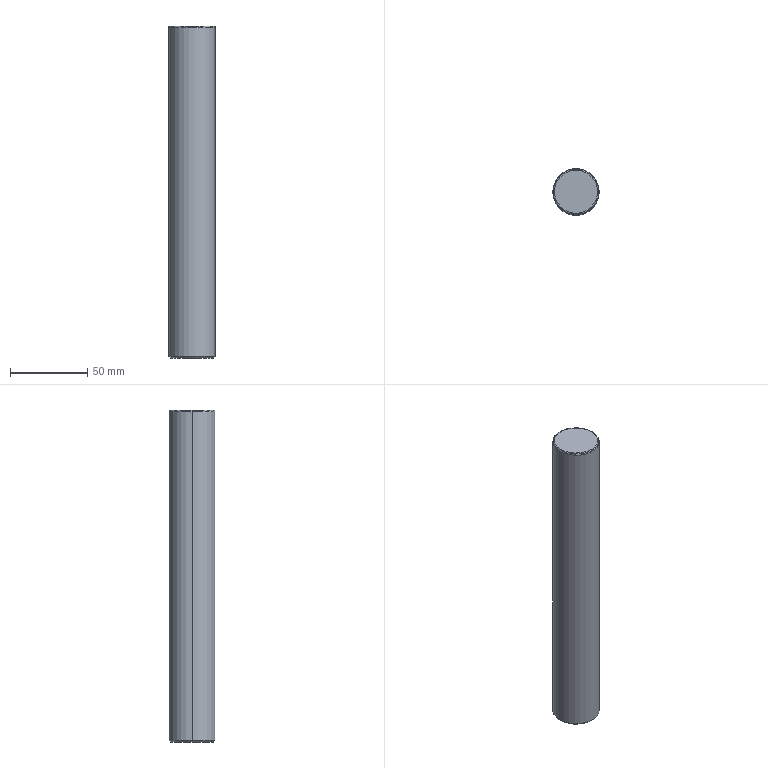Part | Creo | 1 solid | 14 faces | box 30 x 30 x 215 mm | volume 151193 mm3 | cone 4 | cylinder 4 | torus 4 | plane 2 | commonest cylinder face diameters 6.8 x2 30 x2
STEP:
#1=CARTESIAN_POINT('',(-69.,10.,-300.5));
#2=VERTEX_POINT('',#1);
#3=CARTESIAN_POINT('',(-41.,10.,-300.5));
#4=VERTEX_POINT('',#3);
#5=CARTESIAN_POINT('',(-55.,10.,-300.5));
#6=DIRECTION('',(0.,0.,-1.));
#7=DIRECTION('',(-1.,0.,0.));
#8=AXIS2_PLACEMENT_3D('',#5,#6,#7);
#9=CIRCLE('',#8,14.);
#10=EDGE_CURVE('',#2,#4,#9,.T.);
#11=ORIENTED_EDGE('',*,*,#10,.F.);
#12=CARTESIAN_POINT('',(-55.,10.,-300.5));
#13=DIRECTION('',(0.,0.,-1.));
#14=DIRECTION('',(1.,0.,0.));
#15=AXIS2_PLACEMENT_3D('',#12,#13,#14);
#16=CIRCLE('',#15,14.);
#17=EDGE_CURVE('',#4,#2,#16,.T.);
#18=ORIENTED_EDGE('',*,*,#17,.F.);
#19=EDGE_LOOP('',(#11,#18));
#20=FACE_OUTER_BOUND('',#19,.F.);
#21=CARTESIAN_POINT('',(-51.6,10.,-300.5));
#22=VERTEX_POINT('',#21);
#23=CARTESIAN_POINT('',(-58.4,10.,-300.5));
#24=VERTEX_POINT('',#23);
#25=CARTESIAN_POINT('',(-55.,10.,-300.5));
#26=DIRECTION('',(0.,0.,1.));
#27=DIRECTION('',(1.,0.,0.));
#28=AXIS2_PLACEMENT_3D('',#25,#26,#27);
#29=CIRCLE('',#28,3.4);
#30=EDGE_CURVE('',#22,#24,#29,.T.);
#31=ORIENTED_EDGE('',*,*,#30,.F.);
#32=CARTESIAN_POINT('',(-55.,10.,-300.5));
#33=DIRECTION('',(0.,0.,1.));
#34=DIRECTION('',(-1.,0.,0.));
#35=AXIS2_PLACEMENT_3D('',#32,#33,#34);
#36=CIRCLE('',#35,3.4);
#37=EDGE_CURVE('',#24,#22,#36,.T.);
#38=ORIENTED_EDGE('',*,*,#37,.F.);
#39=EDGE_LOOP('',(#31,#38));
#40=FACE_BOUND('',#39,.F.);
#41=CARTESIAN_POINT('',(-55.,10.,-300.5));
#42=DIRECTION('',(0.,0.,-1.));
#43=DIRECTION('',(-1.,0.,0.));
#44=AXIS2_PLACEMENT_3D('',#41,#42,#43);
#45=PLANE('',#44);
#46=ADVANCED_FACE('',(#20,#40),#45,.T.);
#47=ORIENTED_EDGE('',*,*,#10,.T.);
#48=CARTESIAN_POINT('',(-40.,10.,-299.5));
#49=VERTEX_POINT('',#48);
#50=CARTESIAN_POINT('',(-41.,10.,-300.5));
#51=DIRECTION('',(0.7071,0.,0.7071));
#52=VECTOR('',#51,1.414);
#53=LINE('',#50,#52);
#54=EDGE_CURVE('',#4,#49,#53,.T.);
#55=ORIENTED_EDGE('',*,*,#54,.T.);
#56=CARTESIAN_POINT('',(-70.,10.,-299.5));
#57=VERTEX_POINT('',#56);
#58=CARTESIAN_POINT('',(-55.,10.,-299.5));
#59=DIRECTION('',(0.,0.,-1.));
#60=DIRECTION('',(-1.,0.,0.));
#61=AXIS2_PLACEMENT_3D('',#58,#59,#60);
#62=CIRCLE('',#61,15.);
#63=EDGE_CURVE('',#57,#49,#62,.T.);
#64=ORIENTED_EDGE('',*,*,#63,.F.);
#65=CARTESIAN_POINT('',(-69.,10.,-300.5));
#66=DIRECTION('',(-0.7071,0.,0.7071));
#67=VECTOR('',#66,1.414);
#68=LINE('',#65,#67);
#69=EDGE_CURVE('',#2,#57,#68,.T.);
#70=ORIENTED_EDGE('',*,*,#69,.F.);
#71=EDGE_LOOP('',(#47,#55,#64,#70));
#72=FACE_OUTER_BOUND('',#71,.F.);
#73=CARTESIAN_POINT('',(-55.,10.,-300.));
#74=DIRECTION('',(0.,0.,1.));
#75=DIRECTION('',(1.,0.,0.));
#76=AXIS2_PLACEMENT_3D('',#73,#74,#75);
#77=CONICAL_SURFACE('',#76,14.5,45.);
#78=ADVANCED_FACE('',(#72),#77,.T.);
#79=ORIENTED_EDGE('',*,*,#17,.T.);
#80=ORIENTED_EDGE('',*,*,#69,.T.);
#81=CARTESIAN_POINT('',(-55.,10.,-299.5));
#82=DIRECTION('',(0.,0.,-1.));
#83=DIRECTION('',(1.,0.,0.));
#84=AXIS2_PLACEMENT_3D('',#81,#82,#83);
#85=CIRCLE('',#84,15.);
#86=EDGE_CURVE('',#49,#57,#85,.T.);
#87=ORIENTED_EDGE('',*,*,#86,.F.);
#88=ORIENTED_EDGE('',*,*,#54,.F.);
#89=EDGE_LOOP('',(#79,#80,#87,#88));
#90=FACE_OUTER_BOUND('',#89,.F.);
#91=CARTESIAN_POINT('',(-55.,10.,-300.));
#92=DIRECTION('',(0.,0.,1.));
#93=DIRECTION('',(1.,0.,0.));
#94=AXIS2_PLACEMENT_3D('',#91,#92,#93);
#95=CONICAL_SURFACE('',#94,14.5,45.);
#96=ADVANCED_FACE('',(#90),#95,.T.);
#97=ORIENTED_EDGE('',*,*,#86,.T.);
#98=CARTESIAN_POINT('',(-70.,10.,-86.5));
#99=VERTEX_POINT('',#98);
#100=CARTESIAN_POINT('',(-70.,10.,-86.5));
#101=DIRECTION('',(0.,0.,-1.));
#102=VECTOR('',#101,213.);
#103=LINE('',#100,#102);
#104=EDGE_CURVE('',#99,#57,#103,.T.);
#105=ORIENTED_EDGE('',*,*,#104,.F.);
#106=CARTESIAN_POINT('',(-40.,10.,-86.5));
#107=VERTEX_POINT('',#106);
#108=CARTESIAN_POINT('',(-55.,10.,-86.5));
#109=DIRECTION('',(0.,0.,1.));
#110=DIRECTION('',(-1.,0.,0.));
#111=AXIS2_PLACEMENT_3D('',#108,#109,#110);
#112=CIRCLE('',#111,15.);
#113=EDGE_CURVE('',#99,#107,#112,.T.);
#114=ORIENTED_EDGE('',*,*,#113,.T.);
#115=CARTESIAN_POINT('',(-40.,10.,-86.5));
#116=DIRECTION('',(0.,0.,-1.));
#117=VECTOR('',#116,213.);
#118=LINE('',#115,#117);
#119=EDGE_CURVE('',#107,#49,#118,.T.);
#120=ORIENTED_EDGE('',*,*,#119,.T.);
#121=EDGE_LOOP('',(#97,#105,#114,#120));
#122=FACE_OUTER_BOUND('',#121,.F.);
#123=CARTESIAN_POINT('',(-55.,10.,-100.5));
#124=DIRECTION('',(0.,0.,-1.));
#125=DIRECTION('',(-1.,0.,0.));
#126=AXIS2_PLACEMENT_3D('',#123,#124,#125);
#127=CYLINDRICAL_SURFACE('',#126,15.);
#128=ADVANCED_FACE('',(#122),#127,.T.);
#129=ORIENTED_EDGE('',*,*,#63,.T.);
#130=ORIENTED_EDGE('',*,*,#119,.F.);
#131=CARTESIAN_POINT('',(-55.,10.,-86.5));
#132=DIRECTION('',(0.,0.,1.));
#133=DIRECTION('',(1.,0.,0.));
#134=AXIS2_PLACEMENT_3D('',#131,#132,#133);
#135=CIRCLE('',#134,15.);
#136=EDGE_CURVE('',#107,#99,#135,.T.);
#137=ORIENTED_EDGE('',*,*,#136,.T.);
#138=ORIENTED_EDGE('',*,*,#104,.T.);
#139=EDGE_LOOP('',(#129,#130,#137,#138));
#140=FACE_OUTER_BOUND('',#139,.F.);
#141=CARTESIAN_POINT('',(-55.,10.,-100.5));
#142=DIRECTION('',(0.,0.,-1.));
#143=DIRECTION('',(-1.,0.,0.));
#144=AXIS2_PLACEMENT_3D('',#141,#142,#143);
#145=CYLINDRICAL_SURFACE('',#144,15.);
#146=ADVANCED_FACE('',(#140),#145,.T.);
#147=ORIENTED_EDGE('',*,*,#136,.F.);
#148=CARTESIAN_POINT('',(-40.293,10.,-85.793));
#149=VERTEX_POINT('',#148);
#150=CARTESIAN_POINT('',(-41.,10.,-86.5));
#151=DIRECTION('',(0.,-1.,0.));
#152=DIRECTION('',(1.,0.,0.));
#153=AXIS2_PLACEMENT_3D('',#150,#151,#152);
#154=CIRCLE('',#153,1.);
#155=EDGE_CURVE('',#107,#149,#154,.T.);
#156=ORIENTED_EDGE('',*,*,#155,.T.);
#157=CARTESIAN_POINT('',(-69.707,10.,-85.793));
#158=VERTEX_POINT('',#157);
#159=CARTESIAN_POINT('',(-55.,10.,-85.793));
#160=DIRECTION('',(0.,0.,1.));
#161=DIRECTION('',(1.,0.,0.));
#162=AXIS2_PLACEMENT_3D('',#159,#160,#161);
#163=CIRCLE('',#162,14.707);
#164=EDGE_CURVE('',#149,#158,#163,.T.);
#165=ORIENTED_EDGE('',*,*,#164,.T.);
#166=CARTESIAN_POINT('',(-69.,10.,-86.5));
#167=DIRECTION('',(0.,1.,0.));
#168=DIRECTION('',(-1.,0.,0.));
#169=AXIS2_PLACEMENT_3D('',#166,#167,#168);
#170=CIRCLE('',#169,1.);
#171=EDGE_CURVE('',#99,#158,#170,.T.);
#172=ORIENTED_EDGE('',*,*,#171,.F.);
#173=EDGE_LOOP('',(#147,#156,#165,#172));
#174=FACE_OUTER_BOUND('',#173,.F.);
#175=CARTESIAN_POINT('',(-55.,10.,-86.5));
#176=DIRECTION('',(0.,0.,1.));
#177=DIRECTION('',(1.,0.,0.));
#178=AXIS2_PLACEMENT_3D('',#175,#176,#177);
#179=TOROIDAL_SURFACE('',#178,14.,1.);
#180=ADVANCED_FACE('',(#174),#179,.T.);
#181=ORIENTED_EDGE('',*,*,#113,.F.);
#182=ORIENTED_EDGE('',*,*,#171,.T.);
#183=CARTESIAN_POINT('',(-55.,10.,-85.793));
#184=DIRECTION('',(0.,0.,1.));
#185=DIRECTION('',(-1.,0.,0.));
#186=AXIS2_PLACEMENT_3D('',#183,#184,#185);
#187=CIRCLE('',#186,14.707);
#188=EDGE_CURVE('',#158,#149,#187,.T.);
#189=ORIENTED_EDGE('',*,*,#188,.T.);
#190=ORIENTED_EDGE('',*,*,#155,.F.);
#191=EDGE_LOOP('',(#181,#182,#189,#190));
#192=FACE_OUTER_BOUND('',#191,.F.);
#193=CARTESIAN_POINT('',(-55.,10.,-86.5));
#194=DIRECTION('',(0.,0.,1.));
#195=DIRECTION('',(1.,0.,0.));
#196=AXIS2_PLACEMENT_3D('',#193,#194,#195);
#197=TOROIDAL_SURFACE('',#196,14.,1.);
#198=ADVANCED_FACE('',(#192),#197,.T.);
#199=CARTESIAN_POINT('',(-69.,10.,-85.5));
#200=VERTEX_POINT('',#199);
#201=CARTESIAN_POINT('',(-41.,10.,-85.5));
#202=VERTEX_POINT('',#201);
#203=CARTESIAN_POINT('',(-55.,10.,-85.5));
#204=DIRECTION('',(0.,0.,1.));
#205=DIRECTION('',(-1.,0.,0.));
#206=AXIS2_PLACEMENT_3D('',#203,#204,#205);
#207=CIRCLE('',#206,14.);
#208=EDGE_CURVE('',#200,#202,#207,.T.);
#209=ORIENTED_EDGE('',*,*,#208,.T.);
#210=CARTESIAN_POINT('',(-41.,10.,-86.5));
#211=DIRECTION('',(0.,-1.,0.));
#212=DIRECTION('',(0.7071,0.,0.7071));
#213=AXIS2_PLACEMENT_3D('',#210,#211,#212);
#214=CIRCLE('',#213,1.);
#215=EDGE_CURVE('',#149,#202,#214,.T.);
#216=ORIENTED_EDGE('',*,*,#215,.F.);
#217=ORIENTED_EDGE('',*,*,#188,.F.);
#218=CARTESIAN_POINT('',(-69.,10.,-86.5));
#219=DIRECTION('',(0.,1.,0.));
#220=DIRECTION('',(-0.7071,0.,0.7071));
#221=AXIS2_PLACEMENT_3D('',#218,#219,#220);
#222=CIRCLE('',#221,1.);
#223=EDGE_CURVE('',#158,#200,#222,.T.);
#224=ORIENTED_EDGE('',*,*,#223,.T.);
#225=EDGE_LOOP('',(#209,#216,#217,#224));
#226=FACE_OUTER_BOUND('',#225,.F.);
#227=CARTESIAN_POINT('',(-55.,10.,-86.5));
#228=DIRECTION('',(0.,0.,1.));
#229=DIRECTION('',(1.,0.,0.));
#230=AXIS2_PLACEMENT_3D('',#227,#228,#229);
#231=TOROIDAL_SURFACE('',#230,14.,1.);
#232=ADVANCED_FACE('',(#226),#231,.T.);
#233=CARTESIAN_POINT('',(-55.,10.,-85.5));
#234=DIRECTION('',(0.,0.,1.));
#235=DIRECTION('',(1.,0.,0.));
#236=AXIS2_PLACEMENT_3D('',#233,#234,#235);
#237=CIRCLE('',#236,14.);
#238=EDGE_CURVE('',#202,#200,#237,.T.);
#239=ORIENTED_EDGE('',*,*,#238,.F.);
#240=ORIENTED_EDGE('',*,*,#208,.F.);
#241=EDGE_LOOP('',(#239,#240));
#242=FACE_OUTER_BOUND('',#241,.F.);
#243=CARTESIAN_POINT('',(-55.,10.,-85.5));
#244=DIRECTION('',(0.,0.,1.));
#245=DIRECTION('',(1.,0.,0.));
#246=AXIS2_PLACEMENT_3D('',#243,#244,#245);
#247=PLANE('',#246);
#248=ADVANCED_FACE('',(#242),#247,.T.);
#249=ORIENTED_EDGE('',*,*,#238,.T.);
#250=ORIENTED_EDGE('',*,*,#223,.F.);
#251=ORIENTED_EDGE('',*,*,#164,.F.);
#252=ORIENTED_EDGE('',*,*,#215,.T.);
#253=EDGE_LOOP('',(#249,#250,#251,#252));
#254=FACE_OUTER_BOUND('',#253,.F.);
#255=CARTESIAN_POINT('',(-55.,10.,-86.5));
#256=DIRECTION('',(0.,0.,1.));
#257=DIRECTION('',(1.,0.,0.));
#258=AXIS2_PLACEMENT_3D('',#255,#256,#257);
#259=TOROIDAL_SURFACE('',#258,14.,1.);
#260=ADVANCED_FACE('',(#254),#259,.T.);
#261=CARTESIAN_POINT('',(-58.4,10.,-281.463));
#262=VERTEX_POINT('',#261);
#263=CARTESIAN_POINT('',(-51.6,10.,-281.463));
#264=VERTEX_POINT('',#263);
#265=CARTESIAN_POINT('',(-55.,10.,-281.463));
#266=DIRECTION('',(0.,0.,-1.));
#267=DIRECTION('',(-1.,0.,0.));
#268=AXIS2_PLACEMENT_3D('',#265,#266,#267);
#269=CIRCLE('',#268,3.4);
#270=EDGE_CURVE('',#262,#264,#269,.T.);
#271=ORIENTED_EDGE('',*,*,#270,.T.);
#272=CARTESIAN_POINT('',(-51.6,10.,-300.5));
#273=DIRECTION('',(0.,0.,1.));
#274=VECTOR('',#273,19.037);
#275=LINE('',#272,#274);
#276=EDGE_CURVE('',#22,#264,#275,.T.);
#277=ORIENTED_EDGE('',*,*,#276,.F.);
#278=ORIENTED_EDGE('',*,*,#30,.T.);
#279=CARTESIAN_POINT('',(-58.4,10.,-300.5));
#280=DIRECTION('',(0.,0.,1.));
#281=VECTOR('',#280,19.037);
#282=LINE('',#279,#281);
#283=EDGE_CURVE('',#24,#262,#282,.T.);
#284=ORIENTED_EDGE('',*,*,#283,.T.);
#285=EDGE_LOOP('',(#271,#277,#278,#284));
#286=FACE_OUTER_BOUND('',#285,.F.);
#287=CARTESIAN_POINT('',(-55.,10.,-335.5));
#288=DIRECTION('',(0.,0.,1.));
#289=DIRECTION('',(1.,0.,0.));
#290=AXIS2_PLACEMENT_3D('',#287,#288,#289);
#291=CYLINDRICAL_SURFACE('',#290,3.4);
#292=ADVANCED_FACE('',(#286),#291,.F.);
#293=ORIENTED_EDGE('',*,*,#270,.F.);
#294=CARTESIAN_POINT('',(-55.,10.,-279.5));
#295=VERTEX_POINT('',#294);
#296=CARTESIAN_POINT('',(-55.,10.,-279.5));
#297=DIRECTION('',(-0.866,0.,-0.5));
#298=VECTOR('',#297,3.926);
#299=LINE('',#296,#298);
#300=EDGE_CURVE('',#295,#262,#299,.T.);
#301=ORIENTED_EDGE('',*,*,#300,.F.);
#302=CARTESIAN_POINT('',(-55.,10.,-279.5));
#303=DIRECTION('',(0.866,0.,-0.5));
#304=VECTOR('',#303,3.926);
#305=LINE('',#302,#304);
#306=EDGE_CURVE('',#295,#264,#305,.T.);
#307=ORIENTED_EDGE('',*,*,#306,.T.);
#308=EDGE_LOOP('',(#293,#301,#307));
#309=FACE_OUTER_BOUND('',#308,.F.);
#310=CARTESIAN_POINT('',(-55.,10.,-280.547));
#311=DIRECTION('',(0.,0.,-1.));
#312=DIRECTION('',(-1.,0.,0.));
#313=AXIS2_PLACEMENT_3D('',#310,#311,#312);
#314=CONICAL_SURFACE('',#313,1.814,60.);
#315=ADVANCED_FACE('',(#309),#314,.F.);
#316=CARTESIAN_POINT('',(-55.,10.,-281.463));
#317=DIRECTION('',(0.,0.,-1.));
#318=DIRECTION('',(1.,0.,0.));
#319=AXIS2_PLACEMENT_3D('',#316,#317,#318);
#320=CIRCLE('',#319,3.4);
#321=EDGE_CURVE('',#264,#262,#320,.T.);
#322=ORIENTED_EDGE('',*,*,#321,.F.);
#323=ORIENTED_EDGE('',*,*,#306,.F.);
#324=ORIENTED_EDGE('',*,*,#300,.T.);
#325=EDGE_LOOP('',(#322,#323,#324));
#326=FACE_OUTER_BOUND('',#325,.F.);
#327=CARTESIAN_POINT('',(-55.,10.,-280.547));
#328=DIRECTION('',(0.,0.,-1.));
#329=DIRECTION('',(-1.,0.,0.));
#330=AXIS2_PLACEMENT_3D('',#327,#328,#329);
#331=CONICAL_SURFACE('',#330,1.814,60.);
#332=ADVANCED_FACE('',(#326),#331,.F.);
#333=ORIENTED_EDGE('',*,*,#321,.T.);
#334=ORIENTED_EDGE('',*,*,#283,.F.);
#335=ORIENTED_EDGE('',*,*,#37,.T.);
#336=ORIENTED_EDGE('',*,*,#276,.T.);
#337=EDGE_LOOP('',(#333,#334,#335,#336));
#338=FACE_OUTER_BOUND('',#337,.F.);
#339=CARTESIAN_POINT('',(-55.,10.,-335.5));
#340=DIRECTION('',(0.,0.,1.));
#341=DIRECTION('',(1.,0.,0.));
#342=AXIS2_PLACEMENT_3D('',#339,#340,#341);
#343=CYLINDRICAL_SURFACE('',#342,3.4);
#344=ADVANCED_FACE('',(#338),#343,.F.);
#345=CLOSED_SHELL('',(#46,#78,#96,#128,#146,#180,#198,#232,#248,#260,#292,#315,#332,#344));
#346=MANIFOLD_SOLID_BREP('',#345);
#347=(LENGTH_UNIT()NAMED_UNIT(*)SI_UNIT(.MILLI.,.METRE.));
#348=UNCERTAINTY_MEASURE_WITH_UNIT(LENGTH_MEASURE(0.02191),#347,'','');
#349=(NAMED_UNIT(*)PLANE_ANGLE_UNIT()SI_UNIT($,.RADIAN.));
#350=PLANE_ANGLE_MEASURE_WITH_UNIT(PLANE_ANGLE_MEASURE(0.01745),#349);
#351=(CONVERSION_BASED_UNIT('DEGREE',#350)NAMED_UNIT(*)PLANE_ANGLE_UNIT());
#352=(NAMED_UNIT(*)SI_UNIT($,.STERADIAN.)SOLID_ANGLE_UNIT());
#353=(GEOMETRIC_REPRESENTATION_CONTEXT(3)GLOBAL_UNCERTAINTY_ASSIGNED_CONTEXT((#348))GLOBAL_UNIT_ASSIGNED_CONTEXT((#347,#351,#352))REPRESENTATION_CONTEXT('',''));
#354=ADVANCED_BREP_SHAPE_REPRESENTATION('',(#346),#353);